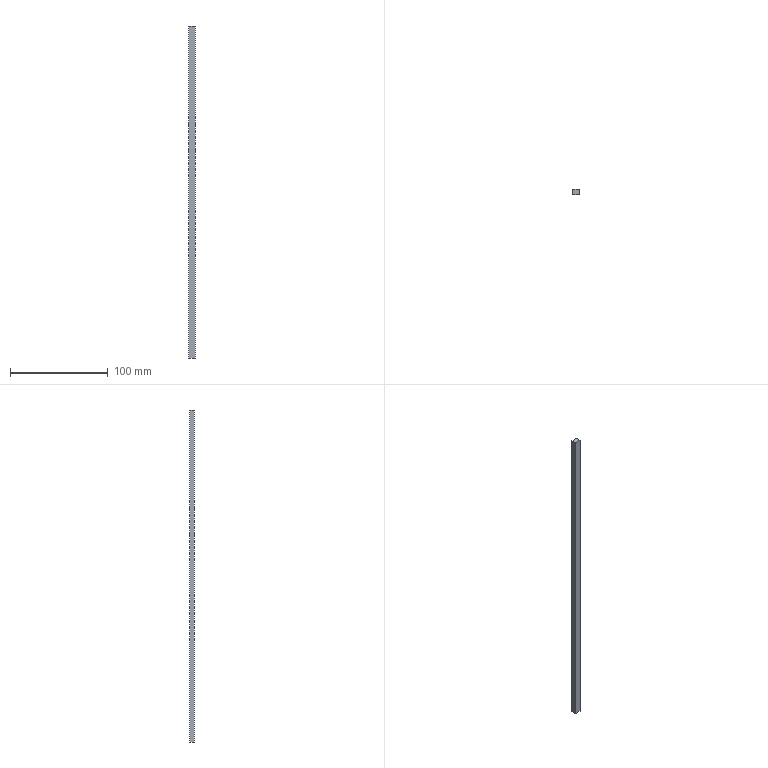Part | SolidWorks | features ICE 2, Extrusion 1, LPattern 1 | 1 solid | 6 faces | box 7 x 4.8 x 340 mm | volume 11424 mm3 | plane 6
STEP:
#1=CARTESIAN_POINT('',(-3.5,2.65,0.));
#2=VERTEX_POINT('',#1);
#3=CARTESIAN_POINT('',(-3.5,-2.15,0.));
#4=VERTEX_POINT('',#3);
#5=CARTESIAN_POINT('',(-3.5,2.65,0.));
#6=DIRECTION('',(0.,-1.,0.));
#7=VECTOR('',#6,1000.);
#8=LINE('',#5,#7);
#9=EDGE_CURVE('',#2,#4,#8,.T.);
#10=ORIENTED_EDGE('',*,*,#9,.T.);
#11=CARTESIAN_POINT('',(-3.5,-2.15,340.));
#12=VERTEX_POINT('',#11);
#13=CARTESIAN_POINT('',(-3.5,-2.15,340.));
#14=DIRECTION('',(0.,0.,-1.));
#15=VECTOR('',#14,1000.);
#16=LINE('',#13,#15);
#17=EDGE_CURVE('',#12,#4,#16,.T.);
#18=ORIENTED_EDGE('',*,*,#17,.F.);
#19=CARTESIAN_POINT('',(-3.5,2.65,340.));
#20=VERTEX_POINT('',#19);
#21=CARTESIAN_POINT('',(-3.5,2.65,340.));
#22=DIRECTION('',(0.,-1.,0.));
#23=VECTOR('',#22,1000.);
#24=LINE('',#21,#23);
#25=EDGE_CURVE('',#20,#12,#24,.T.);
#26=ORIENTED_EDGE('',*,*,#25,.F.);
#27=CARTESIAN_POINT('',(-3.5,2.65,340.));
#28=DIRECTION('',(0.,0.,-1.));
#29=VECTOR('',#28,1000.);
#30=LINE('',#27,#29);
#31=EDGE_CURVE('',#20,#2,#30,.T.);
#32=ORIENTED_EDGE('',*,*,#31,.T.);
#33=EDGE_LOOP('',(#10,#18,#26,#32));
#34=FACE_OUTER_BOUND('',#33,.T.);
#35=CARTESIAN_POINT('',(-3.5,2.65,340.));
#36=DIRECTION('',(1.,0.,0.));
#37=DIRECTION('',(0.,0.,-1.));
#38=AXIS2_PLACEMENT_3D('',#35,#36,#37);
#39=PLANE('',#38);
#40=ADVANCED_FACE('',(#34),#39,.F.);
#41=CARTESIAN_POINT('',(3.5,-2.15,0.));
#42=VERTEX_POINT('',#41);
#43=CARTESIAN_POINT('',(-3.5,-2.15,0.));
#44=DIRECTION('',(1.,0.,0.));
#45=VECTOR('',#44,1000.);
#46=LINE('',#43,#45);
#47=EDGE_CURVE('',#4,#42,#46,.T.);
#48=ORIENTED_EDGE('',*,*,#47,.T.);
#49=CARTESIAN_POINT('',(3.5,-2.15,340.));
#50=VERTEX_POINT('',#49);
#51=CARTESIAN_POINT('',(3.5,-2.15,340.));
#52=DIRECTION('',(0.,0.,-1.));
#53=VECTOR('',#52,1000.);
#54=LINE('',#51,#53);
#55=EDGE_CURVE('',#50,#42,#54,.T.);
#56=ORIENTED_EDGE('',*,*,#55,.F.);
#57=CARTESIAN_POINT('',(-3.5,-2.15,340.));
#58=DIRECTION('',(1.,0.,0.));
#59=VECTOR('',#58,1000.);
#60=LINE('',#57,#59);
#61=EDGE_CURVE('',#12,#50,#60,.T.);
#62=ORIENTED_EDGE('',*,*,#61,.F.);
#63=ORIENTED_EDGE('',*,*,#17,.T.);
#64=EDGE_LOOP('',(#48,#56,#62,#63));
#65=FACE_OUTER_BOUND('',#64,.T.);
#66=CARTESIAN_POINT('',(-3.5,-2.15,340.));
#67=DIRECTION('',(0.,1.,0.));
#68=DIRECTION('',(0.,0.,1.));
#69=AXIS2_PLACEMENT_3D('',#66,#67,#68);
#70=PLANE('',#69);
#71=ADVANCED_FACE('',(#65),#70,.F.);
#72=CARTESIAN_POINT('',(3.5,2.65,0.));
#73=VERTEX_POINT('',#72);
#74=CARTESIAN_POINT('',(3.5,2.65,0.));
#75=DIRECTION('',(0.,-1.,0.));
#76=VECTOR('',#75,1000.);
#77=LINE('',#74,#76);
#78=EDGE_CURVE('',#73,#42,#77,.T.);
#79=ORIENTED_EDGE('',*,*,#78,.F.);
#80=CARTESIAN_POINT('',(3.5,2.65,340.));
#81=VERTEX_POINT('',#80);
#82=CARTESIAN_POINT('',(3.5,2.65,340.));
#83=DIRECTION('',(0.,0.,-1.));
#84=VECTOR('',#83,1000.);
#85=LINE('',#82,#84);
#86=EDGE_CURVE('',#81,#73,#85,.T.);
#87=ORIENTED_EDGE('',*,*,#86,.F.);
#88=CARTESIAN_POINT('',(3.5,2.65,340.));
#89=DIRECTION('',(0.,-1.,0.));
#90=VECTOR('',#89,1000.);
#91=LINE('',#88,#90);
#92=EDGE_CURVE('',#81,#50,#91,.T.);
#93=ORIENTED_EDGE('',*,*,#92,.T.);
#94=ORIENTED_EDGE('',*,*,#55,.T.);
#95=EDGE_LOOP('',(#79,#87,#93,#94));
#96=FACE_OUTER_BOUND('',#95,.T.);
#97=CARTESIAN_POINT('',(3.5,2.65,340.));
#98=DIRECTION('',(1.,0.,0.));
#99=DIRECTION('',(0.,1.,0.));
#100=AXIS2_PLACEMENT_3D('',#97,#98,#99);
#101=PLANE('',#100);
#102=ADVANCED_FACE('',(#96),#101,.T.);
#103=CARTESIAN_POINT('',(-3.5,2.65,0.));
#104=DIRECTION('',(1.,0.,0.));
#105=VECTOR('',#104,1000.);
#106=LINE('',#103,#105);
#107=EDGE_CURVE('',#2,#73,#106,.T.);
#108=ORIENTED_EDGE('',*,*,#107,.F.);
#109=ORIENTED_EDGE('',*,*,#31,.F.);
#110=CARTESIAN_POINT('',(-3.5,2.65,340.));
#111=DIRECTION('',(1.,0.,0.));
#112=VECTOR('',#111,1000.);
#113=LINE('',#110,#112);
#114=EDGE_CURVE('',#20,#81,#113,.T.);
#115=ORIENTED_EDGE('',*,*,#114,.T.);
#116=ORIENTED_EDGE('',*,*,#86,.T.);
#117=EDGE_LOOP('',(#108,#109,#115,#116));
#118=FACE_OUTER_BOUND('',#117,.T.);
#119=CARTESIAN_POINT('',(-3.5,2.65,340.));
#120=DIRECTION('',(0.,1.,0.));
#121=DIRECTION('',(-1.,0.,0.));
#122=AXIS2_PLACEMENT_3D('',#119,#120,#121);
#123=PLANE('',#122);
#124=ADVANCED_FACE('',(#118),#123,.T.);
#125=ORIENTED_EDGE('',*,*,#25,.T.);
#126=ORIENTED_EDGE('',*,*,#61,.T.);
#127=ORIENTED_EDGE('',*,*,#92,.F.);
#128=ORIENTED_EDGE('',*,*,#114,.F.);
#129=EDGE_LOOP('',(#125,#126,#127,#128));
#130=FACE_OUTER_BOUND('',#129,.T.);
#131=CARTESIAN_POINT('',(0.,0.,340.));
#132=DIRECTION('',(0.,0.,1.));
#133=DIRECTION('',(1.,0.,0.));
#134=AXIS2_PLACEMENT_3D('',#131,#132,#133);
#135=PLANE('',#134);
#136=ADVANCED_FACE('',(#130),#135,.T.);
#137=ORIENTED_EDGE('',*,*,#9,.F.);
#138=ORIENTED_EDGE('',*,*,#107,.T.);
#139=ORIENTED_EDGE('',*,*,#78,.T.);
#140=ORIENTED_EDGE('',*,*,#47,.F.);
#141=EDGE_LOOP('',(#137,#138,#139,#140));
#142=FACE_OUTER_BOUND('',#141,.T.);
#143=CARTESIAN_POINT('',(0.,0.,0.));
#144=DIRECTION('',(0.,0.,1.));
#145=DIRECTION('',(1.,0.,0.));
#146=AXIS2_PLACEMENT_3D('',#143,#144,#145);
#147=PLANE('',#146);
#148=ADVANCED_FACE('',(#142),#147,.F.);
#149=CLOSED_SHELL('',(#40,#71,#102,#124,#136,#148));
#150=MANIFOLD_SOLID_BREP('',#149);
#151=CARTESIAN_POINT('',(0.,0.,0.));
#152=DIRECTION('',(0.,0.,1.));
#153=DIRECTION('',(1.,0.,0.));
#154=AXIS2_PLACEMENT_3D('',#151,#152,#153);
#155=(LENGTH_UNIT()NAMED_UNIT(*)SI_UNIT(.MILLI.,.METRE.));
#156=UNCERTAINTY_MEASURE_WITH_UNIT(LENGTH_MEASURE(0.00001),#155,'','');
#157=(NAMED_UNIT(*)PLANE_ANGLE_UNIT()SI_UNIT($,.RADIAN.));
#158=(NAMED_UNIT(*)SI_UNIT($,.STERADIAN.)SOLID_ANGLE_UNIT());
#159=(GEOMETRIC_REPRESENTATION_CONTEXT(3)GLOBAL_UNCERTAINTY_ASSIGNED_CONTEXT((#156))GLOBAL_UNIT_ASSIGNED_CONTEXT((#155,#157,#158))REPRESENTATION_CONTEXT('',''));
#160=ADVANCED_BREP_SHAPE_REPRESENTATION('',(#150,#154),#159);